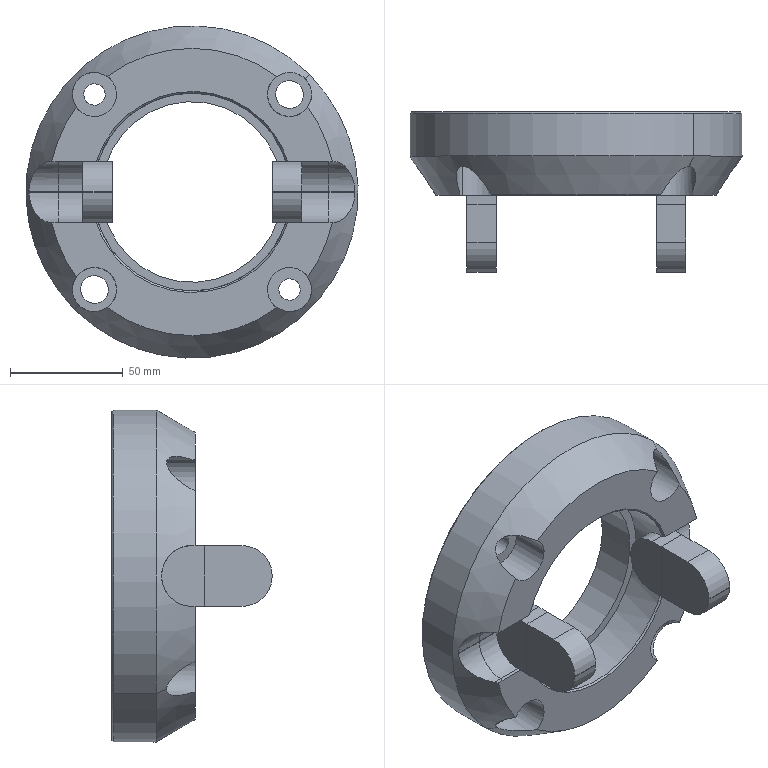Part | SolidWorks | features BaseBody 1 | 1 solid | 87 faces | box 147.154 x 71.054 x 147.154 mm | volume 373178 mm3 | plane 41 | cylinder 38 | cone 8 | commonest cylinder face diameters 26.8 x16 19.595 x8 9.478 x4 12.244 x4 80 x2 87.592 x2